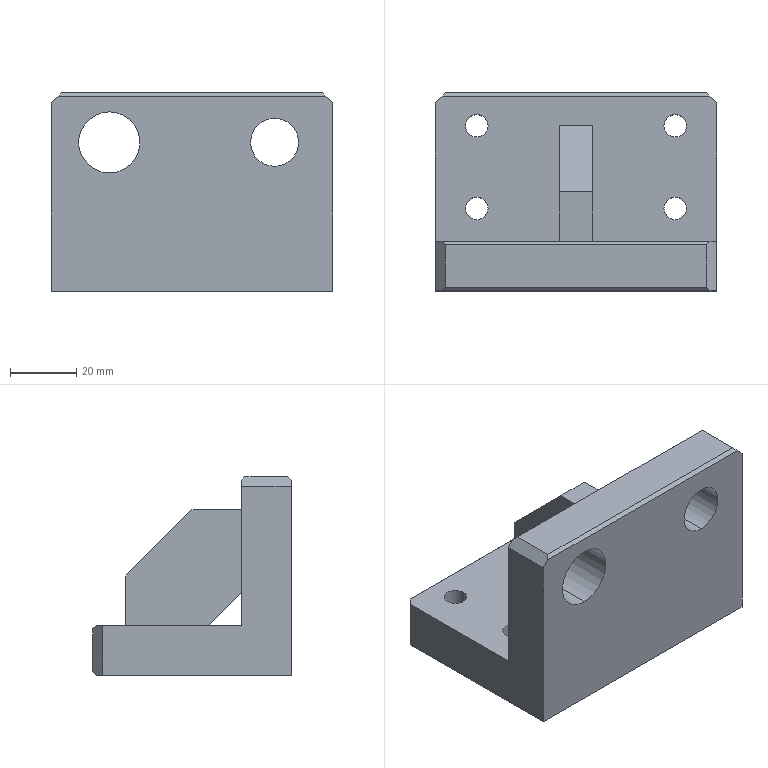Part | STEP file | YCD14007A-08.03.01 Buffer Limit Seat | 1 solid | 34 faces | box 85 x 60 x 60 mm | volume 134508 mm3 | plane 22 | cylinder 12 | commonest cylinder face diameters 6.8 x8 14.5 x2 18.5 x2